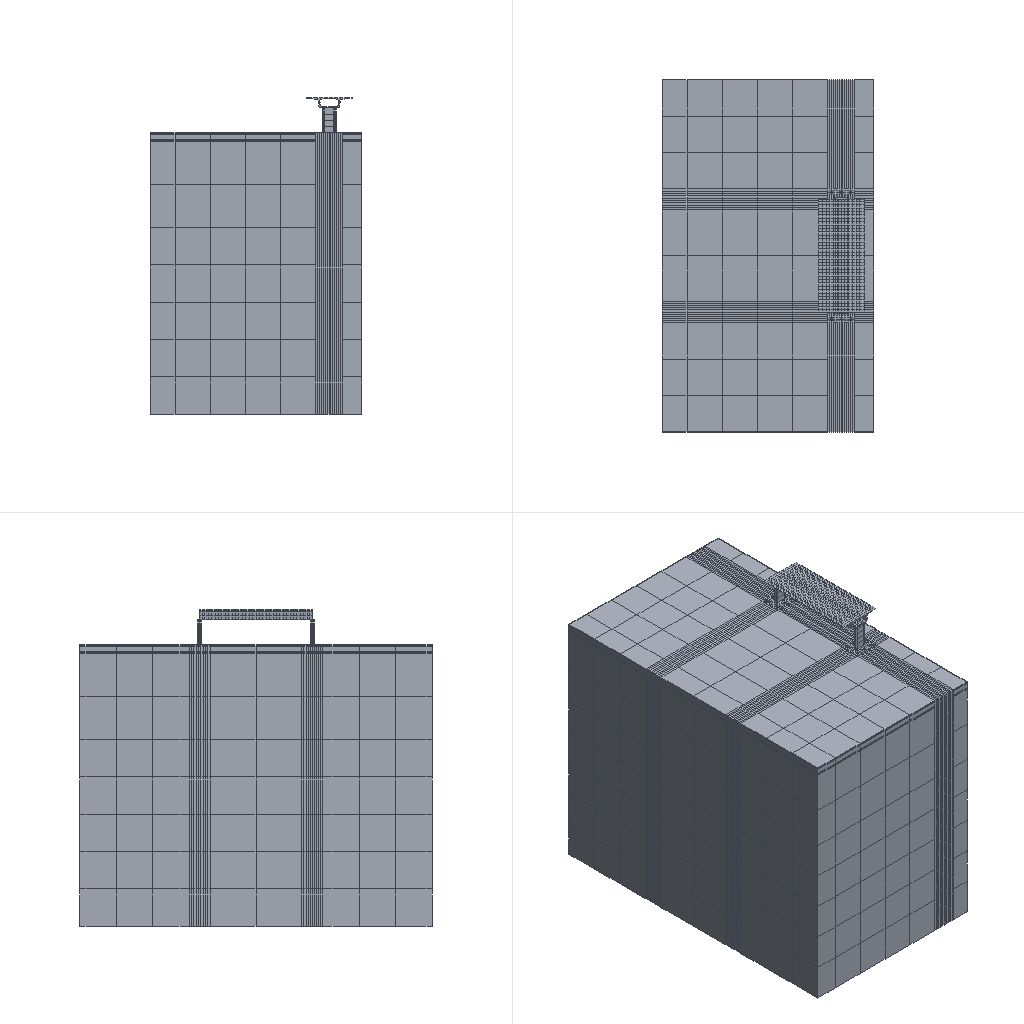Simulation study | abaqus
Set-up summary:
category,name,step,type,value,unit,region
solver,abaqus
solver,version,,,Abaqus/Explicit 2020
units,not stated in the deck,,not stated
analysis,deck,,transient,transient
load_step,Step-1,Step-1,transient
load_step,requested,,,1
mesh,nodes,,,13080
mesh,elements,,,9390
element_type,C3D8R,,solid,9390
load,load commands in deck,,count,1
bc,support commands in deck,,count,3
material,C40,,in results
material,C50,,in results
material,STEEL,,in results
material,T1,,in results
material,T2,,in results
material,T3,,in results
material,T4,,in results
check,setup vs results,,match,"per instance, exact: element labels, types and connectivity; labels of the nodes the elements use; coordinates of those nodes at SINGLE_PRECISION in 4 of 6 instance(s)"
Abaqus input file, long lists of numbers shortened:
*Heading
** Job name: Job-1 Model name: Model-1
** Generated by: Abaqus/CAE 2020
*Preprint, echo=NO, model=NO, history=NO, contact=NO
**
** PARTS
**
*Part, name=asse-1
*Node
      1,           7.,          69.,          80.
      2,           7.,          63.,          80.
** (7891 more lines like these left out)
*Element, type=C3D8R
 1,    8, 1055, 1056,    7,    1, 1032, 1047,    4
 2, 1055, 1054, 1057, 1056, 1032, 1033, 1046, 1047
** (6352 more lines like these left out)
*Nset, nset=Set-1
    1,    2,    3,    4,    5,    6,    7,    8,   17,   18,   19,   20,   37,   38,   41,   42
   52,   53,   54,   55,   56,   57,   58,   75,   76,   77,   78,   79,   80,   98,   99,  100
** (44 more lines like these left out)
*Elset, elset=Set-1
    1,    2,    3,    4,    5,    6,    7,    8,    9,   19,   20,   21,   75,   76,   77,   78
   79,  171,  211,  212,  213,  214,  287,  288,  289,  290,  291,  330,  331,  332,  333,  334
** (16 more lines like these left out)
*Nset, nset=Set-2
    5,    6,    7,    8,   10,   11,   13,   14,   17,   20,   29,   32,   33,   36,   37,   38
   39,   40,   41,   42,   52,   53,   54,   75,   76,   77,   81,   82,   83,   96,   97,   98
** (44 more lines like these left out)
*Elset, elset=Set-2
   22,   23,   24,   25,   26,   27,   28,   29,   30,   40,   41,   42,   43,   44,  172,  210
  215,  216,  217,  315,  316,  317,  320,  321,  322,  323,  324,  325,  326,  327,  328,  329
** (16 more lines like these left out)
*Nset, nset=Set-3
    9,   10,   11,   12,   13,   14,   15,   16,   29,   30,   31,   32,   33,   34,   35,   36
   39,   40,   50,   51,   69,   70,   81,   82,   83,   88,   89,   92,   93,   96,   97,  105
** (44 more lines like these left out)
*Elset, elset=Set-3
   10,   11,   12,   13,   14,   15,   16,   17,   18,   37,   38,   39,   70,   71,   72,   73
   74,  218,  219,  220,  221,  222,  269,  277,  312,  313,  314,  339,  340,  341,  342,  343
** (16 more lines like these left out)
*Nset, nset=Set-4
    9,   12,   15,   16,   21,   22,   23,   24,   25,   26,   27,   28,   30,   31,   34,   35
   43,   44,   45,   46,   47,   48,   49,   50,   51,   59,   60,   61,   62,   63,   64,   65
** (423 more lines like these left out)
*Elset, elset=Set-4
   31,   32,   33,   34,   35,   36,   45,   46,   47,   48,   49,   50,   51,   52,   53,   54
   55,   56,   57,   58,   59,   60,   61,   62,   63,   64,   65,   66,   67,   68,   69,   80
** (344 more lines like these left out)
** Section: t1
*Solid Section, elset=Set-1, material=t1
,
** Section: t3
*Solid Section, elset=Set-3, material=t3
,
** Section: l2
*Solid Section, elset=Set-2, material=t2
,
** Section: t4
*Solid Section, elset=Set-4, material=t4
,
*End Part
**
*Part, name=asse-2
*Node
      1,   57.285,         35.5,   89.7
      2,   56.085,         35.5,   89.7
** (1993 more lines like these left out)
*Element, type=C3D8R
 1,   8,   5, 162, 163,   1,   2, 121, 148
 2, 163, 162, 161, 164, 148, 121, 122, 147
** (1154 more lines like these left out)
*Nset, nset=Set-1, generate
    1,  1995,     1
*Elset, elset=Set-1, generate
    1,  1156,     1
** Section: c50
*Solid Section, elset=Set-1, material=c50
,
*End Part
**
*Part, name=asse-3
*Node
      1,        50.75,          64.,          78.
      2,        51.25,          64.,          78.
** (1222 more lines like these left out)
*Element, type=C3D8R
 1,  558,  126,  554, 1034,  121,    1,  122,  553
 2,  559,  125,  555, 1033,  558,  126,  554, 1034
** (718 more lines like these left out)
*Nset, nset=Set-1, generate
    1,  1224,     1
*Elset, elset=Set-1, generate
   1,  720,    1
** Section: c40
*Solid Section, elset=Set-1, material=c40
,
*End Part
**
*Part, name=asse-4
*Node
      1,   52.15,          34.,   87.1
      2,   52.15,          34.,          87.
** (70 more lines like these left out)
*Element, type=C3D8R
1, 8, 5, 6, 7, 1, 2, 3, 4
2,  1, 12, 13, 14,  2,  9, 10, 11
** (14 more lines like these left out)
*Nset, nset=Set-1, generate
  1,  72,   1
*Elset, elset=Set-1, generate
  1,  16,   1
** Section: steel
*Solid Section, elset=Set-1, material=steel
,
*End Part
**
*Part, name=asse-5
*Node
      1,   52.15,          34.,          87.
      2,   52.15,   34.1,          87.
** (418 more lines like these left out)
*Element, type=C3D8R
1, 118, 124, 119, 113,   1,   2,   3,   4
2, 117, 123, 120, 114, 118, 124, 119, 113
** (254 more lines like these left out)
*Nset, nset=Set-1, generate
   1,  420,    1
*Elset, elset=Set-1, generate
   1,  256,    1
** Section: c50
*Solid Section, elset=Set-1, material=c50
,
*End Part
**
*Part, name=asse-6
*Node
      1,        51.75,          37.,          80.
      2,        51.75,          36.,          80.
** (1474 more lines like these left out)
*Element, type=C3D8R
1, 318, 949, 950, 317,   1, 313, 314,   4
2, 949, 320, 319, 950, 313,   2,   3, 314
** (886 more lines like these left out)
*Nset, nset=Set-1, generate
    1,  1476,     1
*Elset, elset=Set-1, generate
   1,  888,    1
** Section: c40
*Solid Section, elset=Set-1, material=c40
,
*End Part
**
**
** ASSEMBLY
**
*Assembly, name=Assembly
**
*Instance, name=asse-1-1, part=asse-1
*End Instance
**
*Instance, name=asse-2-1, part=asse-2
*End Instance
**
*Instance, name=asse-3-1, part=asse-3
*End Instance
**
*Instance, name=asse-4-1, part=asse-4
*End Instance
**
*Instance, name=asse-5-1, part=asse-5
*End Instance
**
*Instance, name=asse-6-1, part=asse-6
*End Instance
**
*Node
      1,        50.75,          50.,         83.5
*Nset, nset=Set-1, instance=asse-1-1
   17,   18,   19,   20,   21,   22,   23,   24,   29,   30,   31,   32,   84,   85,   86,   87
   88,   89,   90,   91,   98,   99,  102,  103,  104,  105,  111,  113,  121,  122,  123,  137
** (33 more lines like these left out)
*Elset, elset=Set-1, instance=asse-1-1
   19,   31,   32,   37,  173,  176,  179,  182,  185,  188,  191,  194,  197,  212,  215,  225
  228,  256,  259,  262,  265,  268,  314,  315,  348,  360,  361,  366,  371,  376,  532,  535
** (28 more lines like these left out)
*Nset, nset=Set-2, instance=asse-1-1
   45,   46,   48,   49,   53,   54,   56,   57,   63,   64,   67,   68,   69,   70,   73,   74
   76,   77,   79,   80,   82,   83,   85,   87,   89,   91,   97,  104,  105,  106,  107,  108
** (44 more lines like these left out)
*Elset, elset=Set-2, instance=asse-1-1
   45,   46,   47,   48,   49,   50,   51,   52,   53,   54,   55,   56,   57,   58,   59,   60
   61,   62,   63,   64,   65,   66,   67,   68,   69,   75,   76,   77,   78,   79,   90,   91
** (39 more lines like these left out)
*Nset, nset=Set-3, instance=asse-1-1
   43,   44,   45,   46,   65,   66,   67,   68,   90,   91,  115,  116,  117,  121,  122,  128
  129,  135,  169,  170,  171,  184,  185,  186,  187,  203,  204,  212,  214,  215,  218,  228
** (41 more lines like these left out)
*Elset, elset=Set-3, instance=asse-1-1
   45,   46,   47,   48,   49,  126,  127,  128,  129,  130,  131,  132,  133,  134,  197,  198
  199,  229,  230,  231,  232,  233,  254,  255,  256,  274,  286,  382,  383,  384,  385,  386
** (38 more lines like these left out)
*Nset, nset=m_Set-4
 1,
*Elset, elset=_m_Surf-1_S6, internal, instance=asse-2-1
  320,  336,  864,  865,  880,  881, 1130, 1146
*Elset, elset=_m_Surf-1_S4, internal, instance=asse-2-1
  857,  873, 1135, 1151
*Elset, elset=_m_Surf-1_S3, internal, instance=asse-2-1
  314,  330,  592,  593,  608,  609, 1136, 1152
*Elset, elset=_m_Surf-1_S5, internal, instance=asse-2-1
 319, 335, 585, 601
*Surface, type=ELEMENT, name=m_Surf-1
_m_Surf-1_S6, S6
_m_Surf-1_S4, S4
_m_Surf-1_S3, S3
_m_Surf-1_S5, S5
*Elset, elset=_m_Surf-3_S2, internal, instance=asse-6-1
  21,  22,  23,  24,  35,  36,  44,  45,  46,  61,  62,  65,  66,  67,  68,  69
  85,  86,  87,  88,  89,  95,  96,  97,  98,  99, 105, 106, 109, 110, 111, 112
** (14 more lines like these left out)
*Elset, elset=_m_Surf-3_S4, internal, instance=asse-6-1
  18,  32,  42,  52,  54,  55,  56, 166, 168, 169, 190, 192, 193, 200, 202, 203
 204, 215, 220, 228, 238, 240, 241, 242, 252, 254, 295, 312, 314, 319, 352, 359
** (5 more lines like these left out)
*Elset, elset=_m_Surf-3_S3, internal, instance=asse-6-1
  19,  20,  33,  34,  43,  53, 167, 191, 201, 214, 216, 221, 222, 229, 230, 239
 253, 294, 296, 313, 318, 320, 353, 354, 358, 364, 373, 383, 397, 398, 403, 408
** (3 more lines like these left out)
*Elset, elset=_m_Surf-3_S1, internal, instance=asse-6-1
   3,   4,   7,   8,  11,  12,  59,  60,  76,  79,  80,  83,  84, 141, 142, 145
 146, 149, 150, 342, 469, 470, 507, 508, 551, 552, 617, 618, 733, 734
*Surface, type=ELEMENT, name=m_Surf-3
_m_Surf-3_S2, S2
_m_Surf-3_S4, S4
_m_Surf-3_S3, S3
_m_Surf-3_S1, S1
*Elset, elset=_m_Surf-5_S4, internal, instance=asse-6-1
  70,  72,  73,  74,  90, 100, 114, 116, 117, 124, 134, 156, 180, 209, 210, 247
 248, 258, 266, 276, 284, 300, 306, 308, 326, 336, 347, 348, 390, 415, 416, 432
** (3 more lines like these left out)
*Elset, elset=_m_Surf-5_S3, internal, instance=asse-6-1
  71,  91,  92, 101, 102, 115, 125, 126, 127, 128, 135, 136, 157, 158, 181, 182
 183, 184, 208, 246, 259, 260, 267, 277, 285, 286, 301, 302, 307, 327, 337, 338
** (3 more lines like these left out)
*Elset, elset=_m_Surf-5_S2, internal, instance=asse-6-1
   1,   2,   5,   6,   9,  10,  13,  14,  15,  16,  17,  27,  28,  29,  30,  31
  37,  38,  39,  40,  41,  47,  48,  49,  50,  51,  57,  58,  75,  77,  78,  81
** (15 more lines like these left out)
*Elset, elset=_m_Surf-5_S1, internal, instance=asse-6-1
  25,  26,  63,  64, 107, 108, 173, 174, 289, 290, 447, 448, 451, 452, 455, 456
 503, 504, 520, 523, 524, 527, 528, 585, 586, 589, 590, 593, 594, 786
*Surface, type=ELEMENT, name=m_Surf-5
_m_Surf-5_S4, S4
_m_Surf-5_S3, S3
_m_Surf-5_S2, S2
_m_Surf-5_S1, S1
*Elset, elset=_m_Surf-7_S1, internal, instance=asse-5-1
   8,  16,  23,  24,  31,  32,  60,  72,  84,  92, 119, 120, 127, 128, 135, 136
 147, 148, 156, 160, 173, 174, 175, 185, 186, 187, 209, 210, 211, 245, 246, 247
*Elset, elset=_m_Surf-7_S2, internal, instance=asse-5-1
   1,   9,  33,  34,  41,  42,  49,  50,  61,  62,  73,  77,  85,  93,  97,  98
 105, 106, 137, 149, 170, 171, 172, 206, 207, 208, 230, 231, 232, 242, 243, 244
*Surface, type=ELEMENT, name=m_Surf-7
_m_Surf-7_S1, S1
_m_Surf-7_S2, S2
*Elset, elset=_s_Surf-1_S1, internal, instance=asse-4-1
  2, 10, 14
*Elset, elset=_s_Surf-1_S6, internal, instance=asse-4-1
  1,  3,  8,  9, 11, 13, 15
*Elset, elset=_s_Surf-1_S4, internal, instance=asse-4-1
  4,  5,  7, 12, 16
*Elset, elset=_s_Surf-1_S2, internal, instance=asse-4-1
 6,
*Surface, type=ELEMENT, name=s_Surf-1
_s_Surf-1_S1, S1
_s_Surf-1_S6, S6
_s_Surf-1_S4, S4
_s_Surf-1_S2, S2
*Elset, elset=_s_Surf-3_S2, internal, instance=asse-3-1
   1,   3,   5,  16,  18,  20,  31,  33,  35,  46,  48,  50,  61,  63,  65,  76
  78,  80,  91,  93,  95, 106, 108, 110, 121, 123, 125, 136, 138, 140, 151, 153
** (7 more lines like these left out)
*Elset, elset=_s_Surf-3_S3, internal, instance=asse-3-1
 307, 325, 328, 337, 355
*Elset, elset=_s_Surf-3_S4, internal, instance=asse-3-1
 312, 324, 342, 345, 354
*Surface, type=ELEMENT, name=s_Surf-3
_s_Surf-3_S2, S2
_s_Surf-3_S3, S3
_s_Surf-3_S4, S4
*Elset, elset=_s_Surf-5_S2, internal, instance=asse-5-1
   5,  13,  17,  18,  25,  26,  57,  69,  81,  89, 113, 114, 121, 122, 129, 130
 141, 142, 153, 157, 182, 183, 184, 194, 195, 196, 218, 219, 220, 254, 255, 256
*Elset, elset=_s_Surf-5_S1, internal, instance=asse-5-1
   4,  12,  39,  40,  47,  48,  55,  56,  67,  68,  76,  80,  88,  96, 103, 104
 111, 112, 140, 152, 161, 162, 163, 197, 198, 199, 221, 222, 223, 233, 234, 235
*Surface, type=ELEMENT, name=s_Surf-5
_s_Surf-5_S2, S2
_s_Surf-5_S1, S1
*Elset, elset=_s_Surf-7_S6, internal, instance=asse-4-1
  4,  5,  7, 12, 16
*Elset, elset=_s_Surf-7_S4, internal, instance=asse-4-1
  1,  3,  8,  9, 11, 13, 15
*Elset, elset=_s_Surf-7_S2, internal, instance=asse-4-1
  2, 10, 14
*Elset, elset=_s_Surf-7_S1, internal, instance=asse-4-1
 6,
*Surface, type=ELEMENT, name=s_Surf-7
_s_Surf-7_S6, S6
_s_Surf-7_S4, S4
_s_Surf-7_S2, S2
_s_Surf-7_S1, S1
*Elset, elset=_s_Surf-9_S4, internal, instance=asse-1-1
   19,   20,   21,  348,  349,  350,  659,  660,  661,  662,  663,  664,  665,  666,  667,  668
  669,  670,  671,  672,  673,  674,  675,  676, 1867, 1868, 2439, 2747, 2748, 3566, 3567, 3568
** (6 more lines like these left out)
*Elset, elset=_s_Surf-9_S4, internal, instance=asse-2-1
  617,  633,  649,  665,  681,  697,  713,  729,  745,  761,  777,  793,  809,  825,  841,  857
  873,  895,  911,  927,  943,  959,  975,  991, 1007, 1023, 1039, 1055, 1071, 1087, 1103, 1119
** (1 more lines like these left out)
*Elset, elset=_s_Surf-9_S4, internal, instance=asse-5-1
  33,  34,  35,  36,  37,  38,  39,  40,  41,  42,  43,  44,  45,  46,  47,  48
 129, 130, 131, 132, 133, 134, 135, 136, 141, 142, 143, 144, 145, 146, 147, 148
** (1 more lines like these left out)
*Elset, elset=_s_Surf-9_S2, internal, instance=asse-1-1
    1,    2,    3,    4,    5,    6,    7,    8,    9,  287,  288,  289,  290,  291,  330,  331
  332,  333,  334,  335,  336,  337,  338,  572,  573,  574,  575,  576,  712,  713,  714,  715
** (2 more lines like these left out)
*Elset, elset=_s_Surf-9_S1, internal, instance=asse-1-1
   75,   76,   77,   78,   79,  171,  211,  212,  213,  214,  412,  413,  414,  415,  416,  528
  568,  569,  570,  571,  814,  815,  816,  817,  873,  985,  986,  987,  988,  989, 1539, 1540
** (1 more lines like these left out)
*Elset, elset=_s_Surf-9_S6, internal, instance=asse-1-1
 1030, 1031, 1032, 1033, 1034, 1389, 1390, 1619, 2187, 2188, 2459, 2460, 3564, 3565, 4800, 4887
 4888, 4889, 4890, 4891, 4892, 4893, 4894, 4895
*Elset, elset=_s_Surf-9_S6, internal, instance=asse-2-1
   80,   96,  112,  128,  144,  160,  176,  192,  208,  224,  240,  256,  272,  288,  304,  320
  336,  624,  625,  640,  641,  656,  657,  672,  673,  688,  689,  704,  705,  720,  721,  736
** (3 more lines like these left out)
*Elset, elset=_s_Surf-9_S6, internal, instance=asse-5-1
  17,  19,  21,  23,  49,  50,  51,  52,  53,  54,  55,  56,  61,  62,  63,  64
  65,  66,  67,  68, 105, 107, 109, 111, 113, 114, 115, 116, 117, 118, 119, 120
** (2 more lines like these left out)
*Elset, elset=_s_Surf-9_S5, internal, instance=asse-1-1
 1120, 1121, 1122, 1123, 1124, 1125, 1126, 1127, 1128, 1129, 4505, 4506, 4507, 4508, 4509, 4510
 4511, 4512, 4513, 4514, 4709, 4710, 4711, 4712, 4713, 4714, 4715, 4716, 4717
*Elset, elset=_s_Surf-9_S5, internal, instance=asse-2-1
  79,  95, 111, 127, 143, 159, 175, 191, 207, 223, 239, 255, 271, 287, 303, 319
 335, 345, 361, 377, 393, 409, 425, 441, 457, 473, 489, 505, 521, 537, 553, 569
** (1 more lines like these left out)
*Elset, elset=_s_Surf-9_S5, internal, instance=asse-5-1
 161, 164, 167, 170, 245, 248, 251, 254
*Elset, elset=_s_Surf-9_S3, internal, instance=asse-2-1
   74,   90,  106,  122,  138,  154,  170,  186,  202,  218,  234,  250,  266,  282,  298,  314
  330,  352,  353,  368,  369,  384,  385,  400,  401,  416,  417,  432,  433,  448,  449,  464
** (3 more lines like these left out)
*Elset, elset=_s_Surf-9_S3, internal, instance=asse-5-1
  25,  27,  29,  31,  97,  99, 101, 103, 162, 165, 168, 171, 173, 174, 176, 177
 179, 180, 182, 183, 233, 234, 236, 237, 239, 240, 242, 243, 246, 249, 252, 255
*Surface, type=ELEMENT, name=s_Surf-9
_s_Surf-9_S4, S4
_s_Surf-9_S2, S2
_s_Surf-9_S6, S6
_s_Surf-9_S1, S1
_s_Surf-9_S5, S5
_s_Surf-9_S3, S3
*Elset, elset=_s_Surf-10_S5, internal, instance=asse-2-1
   69,   79,   81,   82,   85,   95,   97,   98,  101,  111,  113,  114,  117,  127,  129,  130
  133,  143,  145,  146,  149,  159,  161,  162,  165,  175,  177,  178,  181,  191,  193,  194
** (6 more lines like these left out)
*Elset, elset=_s_Surf-10_S4, internal, instance=asse-2-1
   78,   94,  110,  126,  142,  158,  174,  190,  206,  222,  238,  254,  270,  286,  302,  318
  334,  354,  370,  386,  402,  418,  434,  450,  466,  482,  498,  514,  530,  546,  562,  578
** (6 more lines like these left out)
*Elset, elset=_s_Surf-10_S2, internal, instance=asse-2-1
  1,  2,  3,  4,  5,  6,  7,  8,  9, 10, 11, 12, 13, 14, 15, 16
 17, 20, 21, 22, 23, 24, 25, 26, 27, 28, 29, 30, 31, 32, 33, 34
** (2 more lines like these left out)
*Elset, elset=_s_Surf-10_S6, internal, instance=asse-2-1
   80,   96,  112,  128,  144,  160,  176,  192,  208,  224,  240,  256,  272,  288,  304,  320
  336,  341,  347,  351,  357,  363,  367,  373,  379,  383,  389,  395,  399,  405,  411,  415
** (6 more lines like these left out)
*Elset, elset=_s_Surf-10_S3, internal, instance=asse-2-1
   74,   90,  106,  122,  138,  154,  170,  186,  202,  218,  234,  250,  266,  282,  298,  314
  330,  352,  353,  368,  369,  384,  385,  400,  401,  416,  417,  432,  433,  448,  449,  464
** (6 more lines like these left out)
*Elset, elset=_s_Surf-10_S1, internal, instance=asse-2-1
 18, 19, 50, 51
*Surface, type=ELEMENT, name=s_Surf-10
_s_Surf-10_S5, S5
_s_Surf-10_S4, S4
_s_Surf-10_S2, S2
_s_Surf-10_S6, S6
_s_Surf-10_S3, S3
_s_Surf-10_S1, S1
*Elset, elset=_s_Surf-11_S3, internal, instance=asse-5-1, generate
 25,  31,   2
*Surface, type=ELEMENT, name=s_Surf-11
_s_Surf-11_S3, S3
*Elset, elset=_s_Surf-12_S3, internal, instance=asse-5-1, generate
  97,  103,    2
*Surface, type=ELEMENT, name=s_Surf-12
_s_Surf-12_S3, S3
*Elset, elset=_s_Surf-13_S4, internal, instance=asse-1-1
 1867, 1868, 2439, 2747, 2748, 4610, 4901, 4902, 4903, 4904, 4905
*Elset, elset=_s_Surf-13_S1, internal, instance=asse-1-1
 1539, 1540, 1654, 1655, 2250, 2251, 2357, 2640, 2641, 3162, 3163
*Elset, elset=_s_Surf-13_S6, internal, instance=asse-1-1
 1030, 1031, 1032, 1033, 1034, 1389, 1390, 1619, 2187, 2188, 2459, 2460, 3564, 3565, 4800
*Elset, elset=_s_Surf-13_S2, internal, instance=asse-1-1
 1915, 1916, 2761
*Elset, elset=_s_Surf-13_S5, internal, instance=asse-1-1, generate
 4709,  4717,     1
*Surface, type=ELEMENT, name=s_Surf-13
_s_Surf-13_S4, S4
_s_Surf-13_S1, S1
_s_Surf-13_S6, S6
_s_Surf-13_S2, S2
_s_Surf-13_S5, S5
** Constraint: Constraint-1
*Tie, name=Constraint-1, adjust=yes
s_Surf-1, m_Surf-1
** Constraint: Constraint-2
*Tie, name=Constraint-2, adjust=yes
s_Surf-3, m_Surf-3
** Constraint: Constraint-3
*Tie, name=Constraint-3, adjust=yes
s_Surf-5, m_Surf-5
** Constraint: Constraint-4
*Tie, name=Constraint-4, adjust=yes
s_Surf-7, m_Surf-7
*End Assembly
**
** MATERIALS
**
*Material, name=c40
*Density
2500.,
*Elastic
 3.25e+10, 0.2
*Concrete Damaged Plasticity
36.,    0.1,   1.16, 0.6667,  0.005
*Concrete Compression Hardening
  18760.,          0.
  26800., 0.0007648
 16909.7,  0.002659
 10469.9,  0.004446
 7378.84,  0.006131
 5650.07,   0.007773
 4562.41,   0.009396
 3819.83,   0.01101
 3282.34,   0.01261
 2876.02,   0.01422
*Concrete Tension Stiffening
  2413.9,          0.
   2390., 3.09422e-05
 1263.67, 0.0001701
 815.537, 0.0002883
 615.229, 0.000399
 501.733, 0.000507
  428.08, 0.0006137
 376.039, 0.0007198
 337.082, 0.0008255
 306.681,  0.0009309
 101.338,  0.004176
*Concrete Compression Damage
       0.,          0.
     0.01, 0.0007648
 0.369,  0.002659
 0.6093,  0.004446
  0.7247,  0.006131
 0.8232,   0.007773
 0.8771,   0.009396
  0.9097,   0.01101
 0.9308,   0.01261
 0.9454,   0.01422
*Concrete Tension Damage
       0.,          0.
     0.01, 3.09422e-05
 0.4713, 0.0001701
 0.6588, 0.0002883
 0.7426, 0.000399
 0.8365, 0.000507
 0.8953, 0.0006137
 0.931, 0.0007198
  0.9505, 0.0008255
 0.9624,  0.0009309
 0.999,  0.004176
*Material, name=c50
*Density
2600.,
*Elastic
 3.45e+10, 0.2
*Concrete Damaged Plasticity
40.,    0.1,   1.16, 0.6667,  0.005
*Concrete Compression Hardening
  22680.,          0.
  32400., 0.0007399
 18515.2,  0.002821
 10800.8,  0.004724
 7406.35,  0.006501
 5586.72,  0.008233
  4469.4,  0.009945
  3718.4,   0.01165
 3180.69,   0.01334
 2777.43,   0.01503
*Concrete Tension Stiffening
  2666.4,          0.
   2640., 3.36591e-05
 1264.64, 0.0001837
 786.735, 0.0003077
 584.088, 0.0004238
 472.094,  0.0005372
 400.477, 0.0006495
  350.37,  0.0007611
 313.124,  0.0008724
 284.214, 0.0009834
 92.447,  0.004405
*Concrete Compression Damage
       0.,          0.
     0.01, 0.0007399
 0.4285,  0.002821
 0.6666,  0.004724
 0.7714,  0.006501
 0.8537,  0.008233
 0.8984,  0.009945
   0.9253,   0.01165
 0.9428,   0.01334
 0.9547,   0.01503
*Concrete Tension Damage
       0.,          0.
     0.01, 3.36591e-05
  0.521, 0.0001837
 0.702, 0.0003077
 0.7788, 0.0004238
 0.8612,  0.0005372
 0.9118, 0.0006495
 0.9422,  0.0007611
 0.9587,  0.0008724
 0.9688, 0.0009834
 0.9992,  0.004405
*Material, name=steel
*Density
7800.,
*Elastic
 2.1e+11, 0.3
*Material, name=t1
*Density
1900.,
*Elastic
 1.7e+07, 0.4
*Mohr Coulomb
23., 0.1
*Mohr Coulomb Hardening
24.,0.
*Material, name=t2
*Density
2000.,
*Elastic
 5.6e+07, 0.3
*Mohr Coulomb
42., 0.1
*Mohr Coulomb Hardening
2000.,0.
*Material, name=t3
*Density
2400.,
*Elastic
 6e+08, 0.3
*Mohr Coulomb
40., 0.1
*Mohr Coulomb Hardening
 3e+08,0.
*Material, name=t4
*Density
2600.,
*Elastic
 8e+08, 0.26
*Mohr Coulomb
42., 0.1
*Mohr Coulomb Hardening
 4e+08,0.
**
** INTERACTION PROPERTIES
**
*Surface Interaction, name=IntProp-1
*Friction
 0.2,
*Surface Behavior, pressure-overclosure=HARD
*Incident Wave Interaction Property, name=IntProp-2, type=AIR BLAST
*CONWEP Charge Property
100., 1.
1., 1., 1.
** ----------------------------------------------------------------
**
** STEP: Step-1
**
*Step, name=Step-1, nlgeom=YES
*Dynamic, Explicit
, 0.1
*Bulk Viscosity
0.06, 1.2
**
** BOUNDARY CONDITIONS
**
** Name: BC-1 Type: 位移/转角
*Boundary
Set-1, 2, 2
** Name: BC-2 Type: 位移/转角
*Boundary
Set-2, 1, 1
** Name: BC-3 Type: 位移/转角
*Boundary
Set-3, 3, 3
**
** LOADS
**
** Name: Load-1   Type: Gravity
*Dload
, GRAV, 9.8, 0., 0., -1.
**
** INTERACTIONS
**
** Interaction: Int-1
*Contact, op=NEW
*Contact Inclusions, ALL EXTERIOR
*Contact Property Assignment
 ,  , IntProp-1
** Interaction: Int-2
*Incident Wave Interaction, CONWEP, property=IntProp-2
s_Surf-10, m_Set-4,   , 0., 1.
** Interaction: Int-2-Copy
*Incident Wave Interaction, CONWEP, property=IntProp-2
s_Surf-11, m_Set-4,   , 0., 1.
** Interaction: Int-2-Copy2
*Incident Wave Interaction, CONWEP, property=IntProp-2
s_Surf-12, m_Set-4,   , 0., 1.
** Interaction: Int-2-Copy3
*Incident Wave Interaction, CONWEP, property=IntProp-2
s_Surf-13, m_Set-4,   , 0., 1.
**
** OUTPUT REQUESTS
**
*Restart, write, number interval=1, time marks=NO
**
** FIELD OUTPUT: F-Output-1
**
*Output, field, number interval=50
*Node Output
A, CF, RF, RM, RT, U, V
*Element Output, directions=YES
DAMAGEC, DAMAGET, E, EVF, LE, MISES, MISESMAX, PE, PEEQ, PEEQVAVG, PEVAVG, S, SDEG, SEQUT, SF, SVAVG
YIELDPOT
*Contact Output
CDISP, CSTRESS
**
** HISTORY OUTPUT: H-Output-1
**
*Output, history, variable=PRESELECT, frequency=10
*End Step
Results summary:
result,step,Step-1,completed,increments=7954 time=0.1/0.1
result,analysis,,,transient
result,last_loadstep,,,1
result,primary field,,,U
result,reaction total,,FX,5836260.263,model units
result,reaction total,,FY,-25086.747,model units
result,reaction total,,FZ,9420635181.281,model units